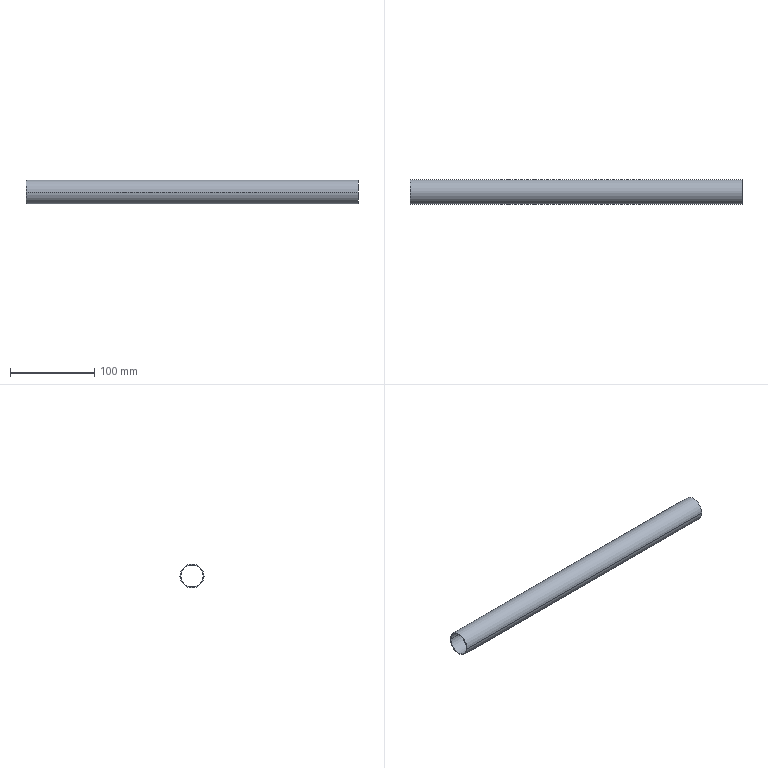Part | STEP file | TUBO REFUERZO LONGITUDINAL.2_Predeterminado<Como mecanizada> | 1 solid | 6 faces | box 395 x 28.6 x 28.6 mm | volume 40802 mm3 | cylinder 4 | plane 2 | commonest cylinder face diameters 26.2 x2 28.6 x2
STEP:
#1=CARTESIAN_POINT('',(-197.5,-14.3,0.));
#2=VERTEX_POINT('',#1);
#3=CARTESIAN_POINT('',(-197.5,14.3,0.));
#4=VERTEX_POINT('',#3);
#5=CARTESIAN_POINT('',(-197.5,0.,0.));
#6=DIRECTION('',(-1.,0.,0.));
#7=DIRECTION('',(0.,-1.,0.));
#8=AXIS2_PLACEMENT_3D('',#5,#6,#7);
#9=CIRCLE('',#8,14.3);
#10=EDGE_CURVE('',#2,#4,#9,.T.);
#11=ORIENTED_EDGE('',*,*,#10,.F.);
#12=CARTESIAN_POINT('',(197.5,-14.3,0.));
#13=VERTEX_POINT('',#12);
#14=CARTESIAN_POINT('',(-197.5,-14.3,0.));
#15=DIRECTION('',(1.,0.,0.));
#16=VECTOR('',#15,1000.);
#17=LINE('',#14,#16);
#18=EDGE_CURVE('',#2,#13,#17,.T.);
#19=ORIENTED_EDGE('',*,*,#18,.T.);
#20=CARTESIAN_POINT('',(197.5,14.3,0.));
#21=VERTEX_POINT('',#20);
#22=CARTESIAN_POINT('',(197.5,0.,0.));
#23=DIRECTION('',(-1.,0.,0.));
#24=DIRECTION('',(0.,-1.,0.));
#25=AXIS2_PLACEMENT_3D('',#22,#23,#24);
#26=CIRCLE('',#25,14.3);
#27=EDGE_CURVE('',#13,#21,#26,.T.);
#28=ORIENTED_EDGE('',*,*,#27,.T.);
#29=CARTESIAN_POINT('',(-197.5,14.3,0.));
#30=DIRECTION('',(1.,0.,0.));
#31=VECTOR('',#30,1000.);
#32=LINE('',#29,#31);
#33=EDGE_CURVE('',#4,#21,#32,.T.);
#34=ORIENTED_EDGE('',*,*,#33,.F.);
#35=EDGE_LOOP('',(#11,#19,#28,#34));
#36=FACE_OUTER_BOUND('',#35,.T.);
#37=CARTESIAN_POINT('',(-197.5,0.,0.));
#38=DIRECTION('',(1.,0.,0.));
#39=DIRECTION('',(0.,1.,0.));
#40=AXIS2_PLACEMENT_3D('',#37,#38,#39);
#41=CYLINDRICAL_SURFACE('',#40,14.3);
#42=ADVANCED_FACE('',(#36),#41,.T.);
#43=CARTESIAN_POINT('',(-197.5,13.1,0.));
#44=VERTEX_POINT('',#43);
#45=CARTESIAN_POINT('',(-197.5,-13.1,0.));
#46=VERTEX_POINT('',#45);
#47=CARTESIAN_POINT('',(-197.5,0.,0.));
#48=DIRECTION('',(-1.,0.,0.));
#49=DIRECTION('',(0.,-1.,0.));
#50=AXIS2_PLACEMENT_3D('',#47,#48,#49);
#51=CIRCLE('',#50,13.1);
#52=EDGE_CURVE('',#44,#46,#51,.T.);
#53=ORIENTED_EDGE('',*,*,#52,.T.);
#54=CARTESIAN_POINT('',(197.5,-13.1,0.));
#55=VERTEX_POINT('',#54);
#56=CARTESIAN_POINT('',(-197.5,-13.1,0.));
#57=DIRECTION('',(1.,0.,0.));
#58=VECTOR('',#57,1000.);
#59=LINE('',#56,#58);
#60=EDGE_CURVE('',#46,#55,#59,.T.);
#61=ORIENTED_EDGE('',*,*,#60,.T.);
#62=CARTESIAN_POINT('',(197.5,13.1,0.));
#63=VERTEX_POINT('',#62);
#64=CARTESIAN_POINT('',(197.5,0.,0.));
#65=DIRECTION('',(-1.,0.,0.));
#66=DIRECTION('',(0.,-1.,0.));
#67=AXIS2_PLACEMENT_3D('',#64,#65,#66);
#68=CIRCLE('',#67,13.1);
#69=EDGE_CURVE('',#63,#55,#68,.T.);
#70=ORIENTED_EDGE('',*,*,#69,.F.);
#71=CARTESIAN_POINT('',(-197.5,13.1,0.));
#72=DIRECTION('',(1.,0.,0.));
#73=VECTOR('',#72,1000.);
#74=LINE('',#71,#73);
#75=EDGE_CURVE('',#44,#63,#74,.T.);
#76=ORIENTED_EDGE('',*,*,#75,.F.);
#77=EDGE_LOOP('',(#53,#61,#70,#76));
#78=FACE_OUTER_BOUND('',#77,.T.);
#79=CARTESIAN_POINT('',(-197.5,0.,0.));
#80=DIRECTION('',(1.,0.,0.));
#81=DIRECTION('',(0.,1.,0.));
#82=AXIS2_PLACEMENT_3D('',#79,#80,#81);
#83=CYLINDRICAL_SURFACE('',#82,13.1);
#84=ADVANCED_FACE('',(#78),#83,.F.);
#85=ORIENTED_EDGE('',*,*,#60,.F.);
#86=CARTESIAN_POINT('',(-197.5,0.,0.));
#87=DIRECTION('',(-1.,0.,0.));
#88=DIRECTION('',(0.,-1.,0.));
#89=AXIS2_PLACEMENT_3D('',#86,#87,#88);
#90=CIRCLE('',#89,13.1);
#91=EDGE_CURVE('',#46,#44,#90,.T.);
#92=ORIENTED_EDGE('',*,*,#91,.T.);
#93=ORIENTED_EDGE('',*,*,#75,.T.);
#94=CARTESIAN_POINT('',(197.5,0.,0.));
#95=DIRECTION('',(-1.,0.,0.));
#96=DIRECTION('',(0.,-1.,0.));
#97=AXIS2_PLACEMENT_3D('',#94,#95,#96);
#98=CIRCLE('',#97,13.1);
#99=EDGE_CURVE('',#55,#63,#98,.T.);
#100=ORIENTED_EDGE('',*,*,#99,.F.);
#101=EDGE_LOOP('',(#85,#92,#93,#100));
#102=FACE_OUTER_BOUND('',#101,.T.);
#103=CARTESIAN_POINT('',(-197.5,0.,0.));
#104=DIRECTION('',(1.,0.,0.));
#105=DIRECTION('',(0.,1.,0.));
#106=AXIS2_PLACEMENT_3D('',#103,#104,#105);
#107=CYLINDRICAL_SURFACE('',#106,13.1);
#108=ADVANCED_FACE('',(#102),#107,.F.);
#109=ORIENTED_EDGE('',*,*,#18,.F.);
#110=CARTESIAN_POINT('',(-197.5,0.,0.));
#111=DIRECTION('',(-1.,0.,0.));
#112=DIRECTION('',(0.,-1.,0.));
#113=AXIS2_PLACEMENT_3D('',#110,#111,#112);
#114=CIRCLE('',#113,14.3);
#115=EDGE_CURVE('',#4,#2,#114,.T.);
#116=ORIENTED_EDGE('',*,*,#115,.F.);
#117=ORIENTED_EDGE('',*,*,#33,.T.);
#118=CARTESIAN_POINT('',(197.5,0.,0.));
#119=DIRECTION('',(-1.,0.,0.));
#120=DIRECTION('',(0.,-1.,0.));
#121=AXIS2_PLACEMENT_3D('',#118,#119,#120);
#122=CIRCLE('',#121,14.3);
#123=EDGE_CURVE('',#21,#13,#122,.T.);
#124=ORIENTED_EDGE('',*,*,#123,.T.);
#125=EDGE_LOOP('',(#109,#116,#117,#124));
#126=FACE_OUTER_BOUND('',#125,.T.);
#127=CARTESIAN_POINT('',(-197.5,0.,0.));
#128=DIRECTION('',(1.,0.,0.));
#129=DIRECTION('',(0.,1.,0.));
#130=AXIS2_PLACEMENT_3D('',#127,#128,#129);
#131=CYLINDRICAL_SURFACE('',#130,14.3);
#132=ADVANCED_FACE('',(#126),#131,.T.);
#133=ORIENTED_EDGE('',*,*,#52,.F.);
#134=ORIENTED_EDGE('',*,*,#91,.F.);
#135=EDGE_LOOP('',(#133,#134));
#136=FACE_BOUND('',#135,.T.);
#137=ORIENTED_EDGE('',*,*,#115,.T.);
#138=ORIENTED_EDGE('',*,*,#10,.T.);
#139=EDGE_LOOP('',(#137,#138));
#140=FACE_OUTER_BOUND('',#139,.T.);
#141=CARTESIAN_POINT('',(-197.5,0.,0.));
#142=DIRECTION('',(-1.,0.,0.));
#143=DIRECTION('',(0.,-1.,0.));
#144=AXIS2_PLACEMENT_3D('',#141,#142,#143);
#145=PLANE('',#144);
#146=ADVANCED_FACE('',(#136,#140),#145,.T.);
#147=ORIENTED_EDGE('',*,*,#69,.T.);
#148=ORIENTED_EDGE('',*,*,#99,.T.);
#149=EDGE_LOOP('',(#147,#148));
#150=FACE_BOUND('',#149,.T.);
#151=ORIENTED_EDGE('',*,*,#123,.F.);
#152=ORIENTED_EDGE('',*,*,#27,.F.);
#153=EDGE_LOOP('',(#151,#152));
#154=FACE_OUTER_BOUND('',#153,.T.);
#155=CARTESIAN_POINT('',(197.5,0.,0.));
#156=DIRECTION('',(-1.,0.,0.));
#157=DIRECTION('',(0.,-1.,0.));
#158=AXIS2_PLACEMENT_3D('',#155,#156,#157);
#159=PLANE('',#158);
#160=ADVANCED_FACE('',(#150,#154),#159,.F.);
#161=CLOSED_SHELL('',(#42,#84,#108,#132,#146,#160));
#162=MANIFOLD_SOLID_BREP('',#161);
#163=CARTESIAN_POINT('',(0.,0.,0.));
#164=DIRECTION('',(0.,0.,1.));
#165=DIRECTION('',(1.,0.,0.));
#166=AXIS2_PLACEMENT_3D('',#163,#164,#165);
#167=(LENGTH_UNIT()NAMED_UNIT(*)SI_UNIT(.MILLI.,.METRE.));
#168=UNCERTAINTY_MEASURE_WITH_UNIT(LENGTH_MEASURE(0.00001),#167,'','');
#169=(NAMED_UNIT(*)PLANE_ANGLE_UNIT()SI_UNIT($,.RADIAN.));
#170=(NAMED_UNIT(*)SI_UNIT($,.STERADIAN.)SOLID_ANGLE_UNIT());
#171=(GEOMETRIC_REPRESENTATION_CONTEXT(3)GLOBAL_UNCERTAINTY_ASSIGNED_CONTEXT((#168))GLOBAL_UNIT_ASSIGNED_CONTEXT((#167,#169,#170))REPRESENTATION_CONTEXT('',''));
#172=ADVANCED_BREP_SHAPE_REPRESENTATION('',(#162,#166),#171);